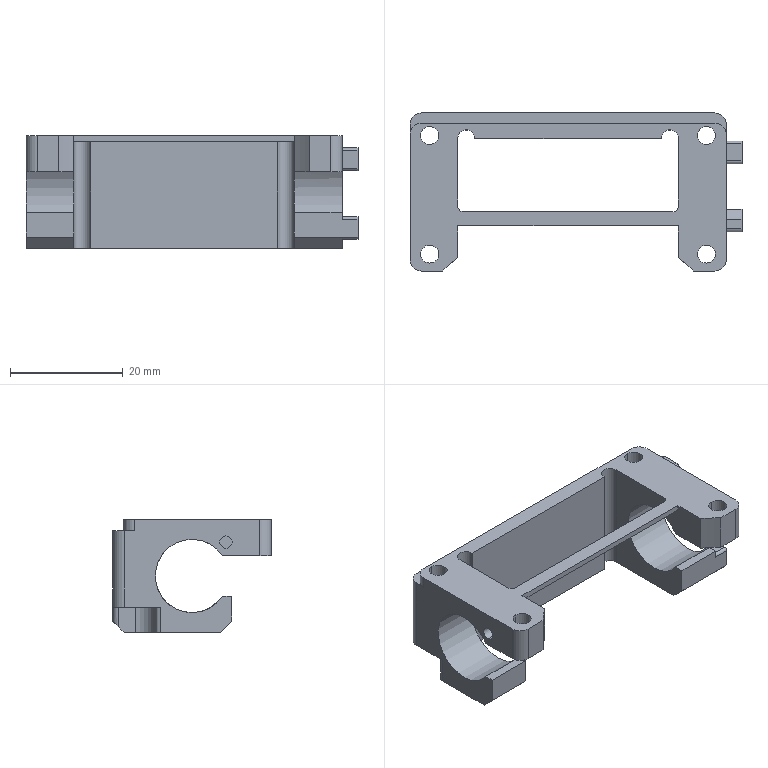Part | 1 solid | 85 faces | box 58.8 x 28 x 20 mm | volume 7782 mm3 | plane 44 | cylinder 41 | commonest cylinder face diameters 3.2 x8 2 x6 4 x6 1 x5 1.8 x4 2.2 x4